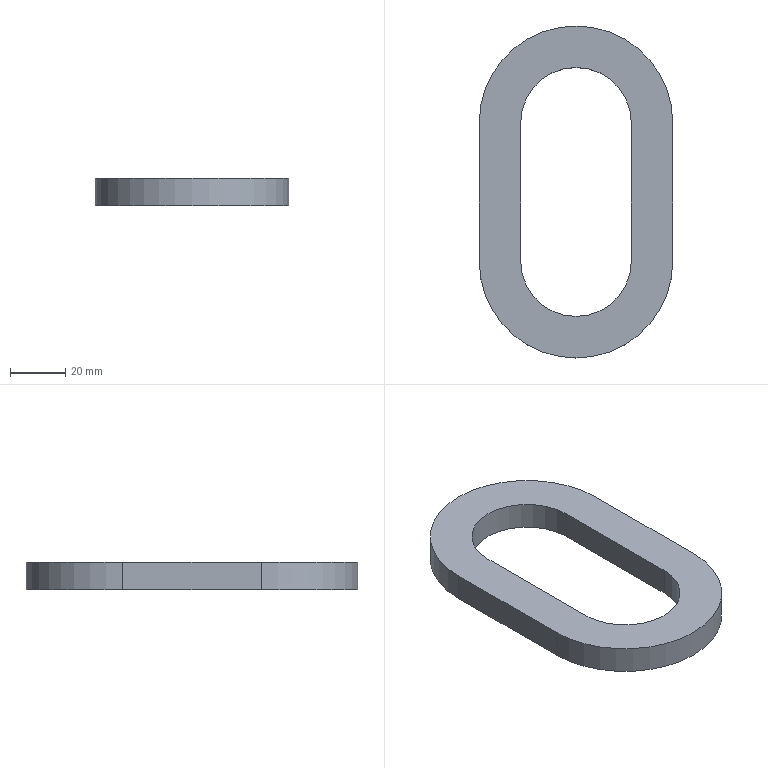Part | SolidWorks | features FlatPattern 1, SMBaseFlange 1, SheetMetal 1 | 1 solid | 10 faces | box 70 x 120 x 10 mm | volume 40918 mm3 | plane 6 | cylinder 4 | commonest cylinder face diameters 40 x2 70 x2
STEP:
#1=CARTESIAN_POINT('',(35.,25.,0.));
#2=VERTEX_POINT('',#1);
#3=CARTESIAN_POINT('',(-35.,25.,0.));
#4=VERTEX_POINT('',#3);
#5=CARTESIAN_POINT('',(0.,25.,0.));
#6=DIRECTION('',(0.,0.,1.));
#7=DIRECTION('',(1.,0.,0.));
#8=AXIS2_PLACEMENT_3D('',#5,#6,#7);
#9=CIRCLE('',#8,35.);
#10=EDGE_CURVE('',#2,#4,#9,.T.);
#11=ORIENTED_EDGE('',*,*,#10,.F.);
#12=CARTESIAN_POINT('',(35.,25.,-10.));
#13=VERTEX_POINT('',#12);
#14=CARTESIAN_POINT('',(35.,25.,-10.));
#15=DIRECTION('',(0.,0.,1.));
#16=VECTOR('',#15,1000.);
#17=LINE('',#14,#16);
#18=EDGE_CURVE('',#13,#2,#17,.T.);
#19=ORIENTED_EDGE('',*,*,#18,.F.);
#20=CARTESIAN_POINT('',(-35.,25.,-10.));
#21=VERTEX_POINT('',#20);
#22=CARTESIAN_POINT('',(0.,25.,-10.));
#23=DIRECTION('',(0.,0.,1.));
#24=DIRECTION('',(1.,0.,0.));
#25=AXIS2_PLACEMENT_3D('',#22,#23,#24);
#26=CIRCLE('',#25,35.);
#27=EDGE_CURVE('',#13,#21,#26,.T.);
#28=ORIENTED_EDGE('',*,*,#27,.T.);
#29=CARTESIAN_POINT('',(-35.,25.,-10.));
#30=DIRECTION('',(0.,0.,1.));
#31=VECTOR('',#30,1000.);
#32=LINE('',#29,#31);
#33=EDGE_CURVE('',#21,#4,#32,.T.);
#34=ORIENTED_EDGE('',*,*,#33,.T.);
#35=EDGE_LOOP('',(#11,#19,#28,#34));
#36=FACE_OUTER_BOUND('',#35,.T.);
#37=CARTESIAN_POINT('',(0.,25.,-10.));
#38=DIRECTION('',(0.,0.,1.));
#39=DIRECTION('',(1.,0.,0.));
#40=AXIS2_PLACEMENT_3D('',#37,#38,#39);
#41=CYLINDRICAL_SURFACE('',#40,35.);
#42=ADVANCED_FACE('',(#36),#41,.T.);
#43=CARTESIAN_POINT('',(35.,-25.,0.));
#44=VERTEX_POINT('',#43);
#45=CARTESIAN_POINT('',(35.,25.,0.));
#46=DIRECTION('',(0.,1.,0.));
#47=VECTOR('',#46,1000.);
#48=LINE('',#45,#47);
#49=EDGE_CURVE('',#44,#2,#48,.T.);
#50=ORIENTED_EDGE('',*,*,#49,.F.);
#51=CARTESIAN_POINT('',(35.,-25.,-10.));
#52=VERTEX_POINT('',#51);
#53=CARTESIAN_POINT('',(35.,-25.,-10.));
#54=DIRECTION('',(0.,0.,1.));
#55=VECTOR('',#54,1000.);
#56=LINE('',#53,#55);
#57=EDGE_CURVE('',#52,#44,#56,.T.);
#58=ORIENTED_EDGE('',*,*,#57,.F.);
#59=CARTESIAN_POINT('',(35.,25.,-10.));
#60=DIRECTION('',(0.,1.,0.));
#61=VECTOR('',#60,1000.);
#62=LINE('',#59,#61);
#63=EDGE_CURVE('',#52,#13,#62,.T.);
#64=ORIENTED_EDGE('',*,*,#63,.T.);
#65=ORIENTED_EDGE('',*,*,#18,.T.);
#66=EDGE_LOOP('',(#50,#58,#64,#65));
#67=FACE_OUTER_BOUND('',#66,.T.);
#68=CARTESIAN_POINT('',(35.,25.,-10.));
#69=DIRECTION('',(1.,0.,0.));
#70=DIRECTION('',(0.,1.,0.));
#71=AXIS2_PLACEMENT_3D('',#68,#69,#70);
#72=PLANE('',#71);
#73=ADVANCED_FACE('',(#67),#72,.T.);
#74=CARTESIAN_POINT('',(-35.,-25.,0.));
#75=VERTEX_POINT('',#74);
#76=CARTESIAN_POINT('',(0.,-25.,0.));
#77=DIRECTION('',(0.,0.,1.));
#78=DIRECTION('',(1.,0.,0.));
#79=AXIS2_PLACEMENT_3D('',#76,#77,#78);
#80=CIRCLE('',#79,35.);
#81=EDGE_CURVE('',#75,#44,#80,.T.);
#82=ORIENTED_EDGE('',*,*,#81,.F.);
#83=CARTESIAN_POINT('',(-35.,-25.,-10.));
#84=VERTEX_POINT('',#83);
#85=CARTESIAN_POINT('',(-35.,-25.,-10.));
#86=DIRECTION('',(0.,0.,1.));
#87=VECTOR('',#86,1000.);
#88=LINE('',#85,#87);
#89=EDGE_CURVE('',#84,#75,#88,.T.);
#90=ORIENTED_EDGE('',*,*,#89,.F.);
#91=CARTESIAN_POINT('',(0.,-25.,-10.));
#92=DIRECTION('',(0.,0.,1.));
#93=DIRECTION('',(1.,0.,0.));
#94=AXIS2_PLACEMENT_3D('',#91,#92,#93);
#95=CIRCLE('',#94,35.);
#96=EDGE_CURVE('',#84,#52,#95,.T.);
#97=ORIENTED_EDGE('',*,*,#96,.T.);
#98=ORIENTED_EDGE('',*,*,#57,.T.);
#99=EDGE_LOOP('',(#82,#90,#97,#98));
#100=FACE_OUTER_BOUND('',#99,.T.);
#101=CARTESIAN_POINT('',(0.,-25.,-10.));
#102=DIRECTION('',(0.,0.,1.));
#103=DIRECTION('',(1.,0.,0.));
#104=AXIS2_PLACEMENT_3D('',#101,#102,#103);
#105=CYLINDRICAL_SURFACE('',#104,35.);
#106=ADVANCED_FACE('',(#100),#105,.T.);
#107=CARTESIAN_POINT('',(-35.,25.,0.));
#108=DIRECTION('',(0.,-1.,0.));
#109=VECTOR('',#108,1000.);
#110=LINE('',#107,#109);
#111=EDGE_CURVE('',#4,#75,#110,.T.);
#112=ORIENTED_EDGE('',*,*,#111,.F.);
#113=ORIENTED_EDGE('',*,*,#33,.F.);
#114=CARTESIAN_POINT('',(-35.,25.,-10.));
#115=DIRECTION('',(0.,-1.,0.));
#116=VECTOR('',#115,1000.);
#117=LINE('',#114,#116);
#118=EDGE_CURVE('',#21,#84,#117,.T.);
#119=ORIENTED_EDGE('',*,*,#118,.T.);
#120=ORIENTED_EDGE('',*,*,#89,.T.);
#121=EDGE_LOOP('',(#112,#113,#119,#120));
#122=FACE_OUTER_BOUND('',#121,.T.);
#123=CARTESIAN_POINT('',(-35.,25.,-10.));
#124=DIRECTION('',(-1.,0.,0.));
#125=DIRECTION('',(0.,-1.,0.));
#126=AXIS2_PLACEMENT_3D('',#123,#124,#125);
#127=PLANE('',#126);
#128=ADVANCED_FACE('',(#122),#127,.T.);
#129=CARTESIAN_POINT('',(20.,-25.,-10.));
#130=VERTEX_POINT('',#129);
#131=CARTESIAN_POINT('',(20.,25.,-10.));
#132=VERTEX_POINT('',#131);
#133=CARTESIAN_POINT('',(20.,25.,-10.));
#134=DIRECTION('',(0.,1.,0.));
#135=VECTOR('',#134,1000.);
#136=LINE('',#133,#135);
#137=EDGE_CURVE('',#130,#132,#136,.T.);
#138=ORIENTED_EDGE('',*,*,#137,.T.);
#139=CARTESIAN_POINT('',(-20.,25.,-10.));
#140=VERTEX_POINT('',#139);
#141=CARTESIAN_POINT('',(0.,25.,-10.));
#142=DIRECTION('',(0.,0.,1.));
#143=DIRECTION('',(1.,0.,0.));
#144=AXIS2_PLACEMENT_3D('',#141,#142,#143);
#145=CIRCLE('',#144,20.);
#146=EDGE_CURVE('',#132,#140,#145,.T.);
#147=ORIENTED_EDGE('',*,*,#146,.T.);
#148=CARTESIAN_POINT('',(-20.,-25.,-10.));
#149=VERTEX_POINT('',#148);
#150=CARTESIAN_POINT('',(-20.,25.,-10.));
#151=DIRECTION('',(0.,-1.,0.));
#152=VECTOR('',#151,1000.);
#153=LINE('',#150,#152);
#154=EDGE_CURVE('',#140,#149,#153,.T.);
#155=ORIENTED_EDGE('',*,*,#154,.T.);
#156=CARTESIAN_POINT('',(0.,-25.,-10.));
#157=DIRECTION('',(0.,0.,1.));
#158=DIRECTION('',(1.,0.,0.));
#159=AXIS2_PLACEMENT_3D('',#156,#157,#158);
#160=CIRCLE('',#159,20.);
#161=EDGE_CURVE('',#149,#130,#160,.T.);
#162=ORIENTED_EDGE('',*,*,#161,.T.);
#163=EDGE_LOOP('',(#138,#147,#155,#162));
#164=FACE_BOUND('',#163,.T.);
#165=ORIENTED_EDGE('',*,*,#27,.F.);
#166=ORIENTED_EDGE('',*,*,#63,.F.);
#167=ORIENTED_EDGE('',*,*,#96,.F.);
#168=ORIENTED_EDGE('',*,*,#118,.F.);
#169=EDGE_LOOP('',(#165,#166,#167,#168));
#170=FACE_OUTER_BOUND('',#169,.T.);
#171=CARTESIAN_POINT('',(0.,25.,-10.));
#172=DIRECTION('',(0.,0.,1.));
#173=DIRECTION('',(1.,0.,0.));
#174=AXIS2_PLACEMENT_3D('',#171,#172,#173);
#175=PLANE('',#174);
#176=ADVANCED_FACE('',(#164,#170),#175,.F.);
#177=CARTESIAN_POINT('',(20.,25.,0.));
#178=VERTEX_POINT('',#177);
#179=CARTESIAN_POINT('',(-20.,25.,0.));
#180=VERTEX_POINT('',#179);
#181=CARTESIAN_POINT('',(0.,25.,0.));
#182=DIRECTION('',(0.,0.,1.));
#183=DIRECTION('',(1.,0.,0.));
#184=AXIS2_PLACEMENT_3D('',#181,#182,#183);
#185=CIRCLE('',#184,20.);
#186=EDGE_CURVE('',#178,#180,#185,.T.);
#187=ORIENTED_EDGE('',*,*,#186,.F.);
#188=CARTESIAN_POINT('',(20.,-25.,0.));
#189=VERTEX_POINT('',#188);
#190=CARTESIAN_POINT('',(20.,25.,0.));
#191=DIRECTION('',(0.,1.,0.));
#192=VECTOR('',#191,1000.);
#193=LINE('',#190,#192);
#194=EDGE_CURVE('',#189,#178,#193,.T.);
#195=ORIENTED_EDGE('',*,*,#194,.F.);
#196=CARTESIAN_POINT('',(-20.,-25.,0.));
#197=VERTEX_POINT('',#196);
#198=CARTESIAN_POINT('',(0.,-25.,0.));
#199=DIRECTION('',(0.,0.,1.));
#200=DIRECTION('',(1.,0.,0.));
#201=AXIS2_PLACEMENT_3D('',#198,#199,#200);
#202=CIRCLE('',#201,20.);
#203=EDGE_CURVE('',#197,#189,#202,.T.);
#204=ORIENTED_EDGE('',*,*,#203,.F.);
#205=CARTESIAN_POINT('',(-20.,25.,0.));
#206=DIRECTION('',(0.,-1.,0.));
#207=VECTOR('',#206,1000.);
#208=LINE('',#205,#207);
#209=EDGE_CURVE('',#180,#197,#208,.T.);
#210=ORIENTED_EDGE('',*,*,#209,.F.);
#211=EDGE_LOOP('',(#187,#195,#204,#210));
#212=FACE_BOUND('',#211,.T.);
#213=ORIENTED_EDGE('',*,*,#10,.T.);
#214=ORIENTED_EDGE('',*,*,#111,.T.);
#215=ORIENTED_EDGE('',*,*,#81,.T.);
#216=ORIENTED_EDGE('',*,*,#49,.T.);
#217=EDGE_LOOP('',(#213,#214,#215,#216));
#218=FACE_OUTER_BOUND('',#217,.T.);
#219=CARTESIAN_POINT('',(0.,25.,0.));
#220=DIRECTION('',(0.,0.,1.));
#221=DIRECTION('',(1.,0.,0.));
#222=AXIS2_PLACEMENT_3D('',#219,#220,#221);
#223=PLANE('',#222);
#224=ADVANCED_FACE('',(#212,#218),#223,.T.);
#225=ORIENTED_EDGE('',*,*,#186,.T.);
#226=CARTESIAN_POINT('',(-20.,25.,-10.));
#227=DIRECTION('',(0.,0.,1.));
#228=VECTOR('',#227,1000.);
#229=LINE('',#226,#228);
#230=EDGE_CURVE('',#140,#180,#229,.T.);
#231=ORIENTED_EDGE('',*,*,#230,.F.);
#232=ORIENTED_EDGE('',*,*,#146,.F.);
#233=CARTESIAN_POINT('',(20.,25.,-10.));
#234=DIRECTION('',(0.,0.,1.));
#235=VECTOR('',#234,1000.);
#236=LINE('',#233,#235);
#237=EDGE_CURVE('',#132,#178,#236,.T.);
#238=ORIENTED_EDGE('',*,*,#237,.T.);
#239=EDGE_LOOP('',(#225,#231,#232,#238));
#240=FACE_OUTER_BOUND('',#239,.T.);
#241=CARTESIAN_POINT('',(0.,25.,-10.));
#242=DIRECTION('',(0.,0.,1.));
#243=DIRECTION('',(1.,0.,0.));
#244=AXIS2_PLACEMENT_3D('',#241,#242,#243);
#245=CYLINDRICAL_SURFACE('',#244,20.);
#246=ADVANCED_FACE('',(#240),#245,.F.);
#247=ORIENTED_EDGE('',*,*,#194,.T.);
#248=ORIENTED_EDGE('',*,*,#237,.F.);
#249=ORIENTED_EDGE('',*,*,#137,.F.);
#250=CARTESIAN_POINT('',(20.,-25.,-10.));
#251=DIRECTION('',(0.,0.,1.));
#252=VECTOR('',#251,1000.);
#253=LINE('',#250,#252);
#254=EDGE_CURVE('',#130,#189,#253,.T.);
#255=ORIENTED_EDGE('',*,*,#254,.T.);
#256=EDGE_LOOP('',(#247,#248,#249,#255));
#257=FACE_OUTER_BOUND('',#256,.T.);
#258=CARTESIAN_POINT('',(20.,25.,-10.));
#259=DIRECTION('',(1.,0.,0.));
#260=DIRECTION('',(0.,1.,0.));
#261=AXIS2_PLACEMENT_3D('',#258,#259,#260);
#262=PLANE('',#261);
#263=ADVANCED_FACE('',(#257),#262,.F.);
#264=ORIENTED_EDGE('',*,*,#203,.T.);
#265=ORIENTED_EDGE('',*,*,#254,.F.);
#266=ORIENTED_EDGE('',*,*,#161,.F.);
#267=CARTESIAN_POINT('',(-20.,-25.,-10.));
#268=DIRECTION('',(0.,0.,1.));
#269=VECTOR('',#268,1000.);
#270=LINE('',#267,#269);
#271=EDGE_CURVE('',#149,#197,#270,.T.);
#272=ORIENTED_EDGE('',*,*,#271,.T.);
#273=EDGE_LOOP('',(#264,#265,#266,#272));
#274=FACE_OUTER_BOUND('',#273,.T.);
#275=CARTESIAN_POINT('',(0.,-25.,-10.));
#276=DIRECTION('',(0.,0.,1.));
#277=DIRECTION('',(1.,0.,0.));
#278=AXIS2_PLACEMENT_3D('',#275,#276,#277);
#279=CYLINDRICAL_SURFACE('',#278,20.);
#280=ADVANCED_FACE('',(#274),#279,.F.);
#281=ORIENTED_EDGE('',*,*,#209,.T.);
#282=ORIENTED_EDGE('',*,*,#271,.F.);
#283=ORIENTED_EDGE('',*,*,#154,.F.);
#284=ORIENTED_EDGE('',*,*,#230,.T.);
#285=EDGE_LOOP('',(#281,#282,#283,#284));
#286=FACE_OUTER_BOUND('',#285,.T.);
#287=CARTESIAN_POINT('',(-20.,25.,-10.));
#288=DIRECTION('',(-1.,0.,0.));
#289=DIRECTION('',(0.,-1.,0.));
#290=AXIS2_PLACEMENT_3D('',#287,#288,#289);
#291=PLANE('',#290);
#292=ADVANCED_FACE('',(#286),#291,.F.);
#293=CLOSED_SHELL('',(#42,#73,#106,#128,#176,#224,#246,#263,#280,#292));
#294=MANIFOLD_SOLID_BREP('',#293);
#295=CARTESIAN_POINT('',(0.,0.,0.));
#296=DIRECTION('',(0.,0.,1.));
#297=DIRECTION('',(1.,0.,0.));
#298=AXIS2_PLACEMENT_3D('',#295,#296,#297);
#299=(LENGTH_UNIT()NAMED_UNIT(*)SI_UNIT(.MILLI.,.METRE.));
#300=UNCERTAINTY_MEASURE_WITH_UNIT(LENGTH_MEASURE(0.00001),#299,'','');
#301=(NAMED_UNIT(*)PLANE_ANGLE_UNIT()SI_UNIT($,.RADIAN.));
#302=(NAMED_UNIT(*)SI_UNIT($,.STERADIAN.)SOLID_ANGLE_UNIT());
#303=(GEOMETRIC_REPRESENTATION_CONTEXT(3)GLOBAL_UNCERTAINTY_ASSIGNED_CONTEXT((#300))GLOBAL_UNIT_ASSIGNED_CONTEXT((#299,#301,#302))REPRESENTATION_CONTEXT('',''));
#304=ADVANCED_BREP_SHAPE_REPRESENTATION('',(#294,#298),#303);